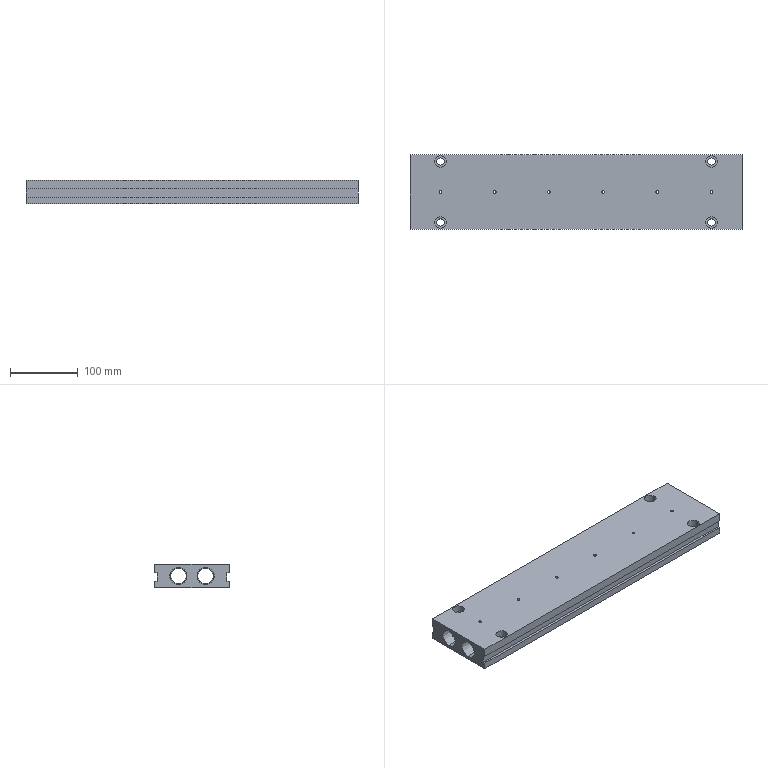Part | STEP file | LM-05-1227_default | 1 solid | 62 faces | box 490 x 110 x 35 mm | volume 1412301 mm3 | cylinder 32 | plane 22 | cone 8 | commonest cylinder face diameters 4 x12 11 x8 17 x8 23 x4